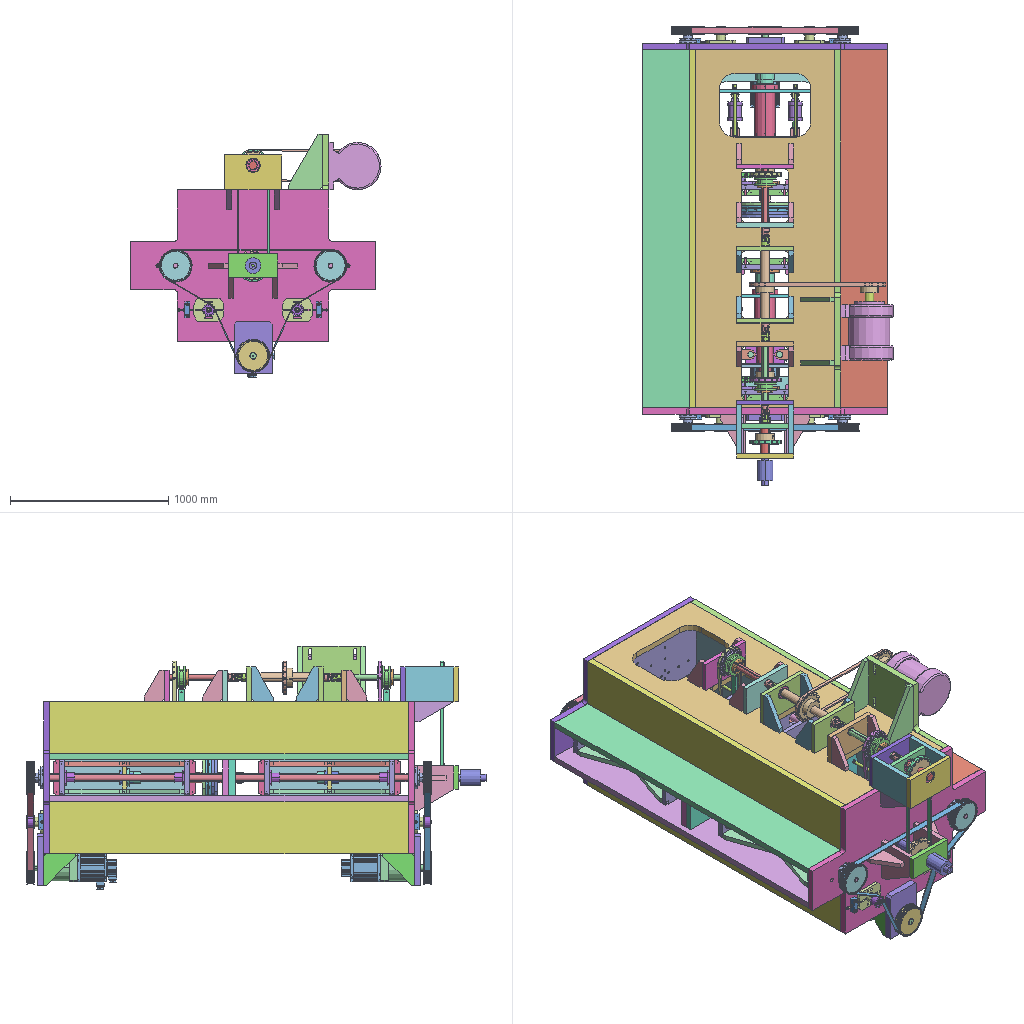Assembly | SolidWorks | 129 different items | 522 placed | box 1583 x 2910 x 1538 mm
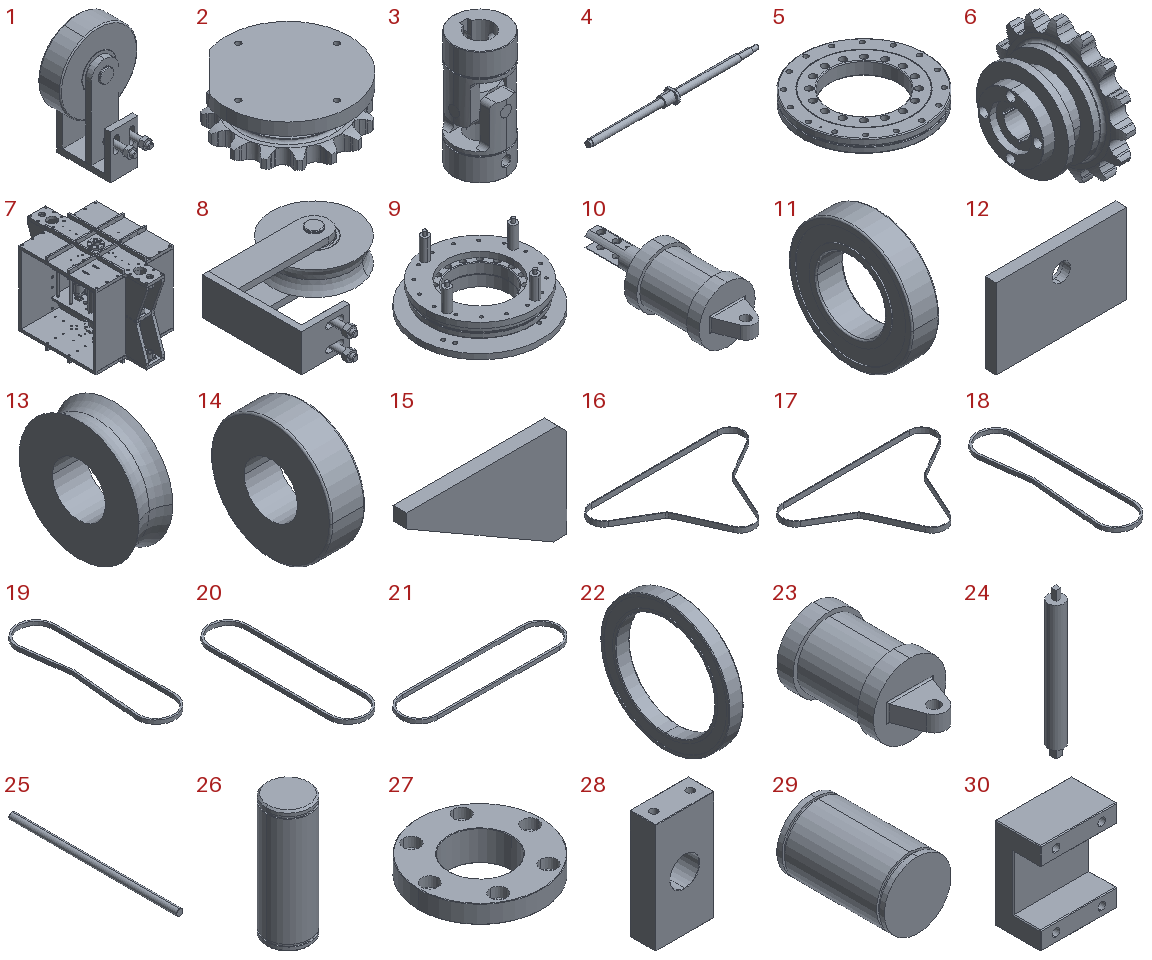Parts list (item | name | quantity | parent item | size | volume | features):
1 | (subassembly) | x2 | - | 140 x 135.4 x 210 mm | 1382662 mm3 | features ReferencePattern 2, LocalLPattern 1
2 | (subassembly) | x2 | - | 200 x 200 x 79.02 mm | 1384453 mm3 | -
3 | (subassembly) | x3 | - | 50 x 50 x 108 mm | 130894 mm3 | -
4 | (subassembly) | x4 | - | 1281 x 110 x 85 mm | 2659708 mm3 | -
5 | (subassembly) | x1 | in 9 | 380 x 380 x 40 mm | 2781012 mm3 | features ReferencePattern 29, CompositeCurve 5, LocalCirPattern 1, MirrorCompFeat 1
6 | (subassembly) | x2 | - | 100.469 x 197.46 x 198.492 mm | 1236352 mm3 | -
7 | (subassembly) | x2 | - | - | 136371359 mm3 | -
8 | (subassembly) | x2 | - | 230 x 244.4 x 70 mm | 814861 mm3 | features ReferencePattern 2, LocalLPattern 1
9 | (subassembly) | x1 | - | 460 x 460 x 195 mm | 7776901 mm3 | features InContextFeatHolder 6, ReferencePattern 3, LocalCirPattern 1
10 | (subassembly) | x4 | in 7 | 90 x 260 x 90 mm | 556632 mm3 | -
11 | - | x4 | - | 20 x 90 x 90 mm | 83545 mm3 | features Fillet 2, Revolution 1
12 | - | x1 | - | 360 x 30 x 220 mm | 2312972 mm3 | features Cut 2, Extrusion 1
13 | - | x2 | in 8 | 40 x 140 x 140 mm | 406899 mm3 | features ICE 1, Revolution 1
14 | - | x4 | in 1 | 40 x 140 x 140 mm | 494239 mm3 | features Fillet 1, ICE 1, Revolution 1
15 | - | x2 | - | 350 x 30 x 214.752 mm | 1362087 mm3 | features Extrusion 1
16 | - | x1 | - | 1186 x 775.76 x 38 mm | 604622 mm3 | features BeltProfileFeature 1, ExtruThin 1
17 | - | x1 | - | 1186 x 775.76 x 38 mm | 604622 mm3 | features BeltProfileFeature 1, ExtruThin 1
18 | - | x1 | - | 203.25 x 838.25 x 20 mm | 376153 mm3 | features BeltProfileFeature 1, ExtruThin 1
19 | - | x1 | - | 203.25 x 838.25 x 20 mm | 376153 mm3 | features BeltProfileFeature 1, ExtruThin 1
20 | - | x1 | - | 203.25 x 838.25 x 20 mm | 375423 mm3 | features BeltProfileFeature 1, ExtruThin 1
21 | - | x1 | - | 863.25 x 208.25 x 20 mm | 385430 mm3 | features BeltProfileFeature 1, ExtruThin 1
22 | - | x4 | in 2 | 7 x 65 x 65 mm | 8944 mm3 | features Fillet 2, Revolution 1
23 | - | x4 | in 10 | 90 x 165 x 90 mm | 446114 mm3 | features ICE 5, Extrusion 1, Fillet 1
24 | - | x1 | - | 50 x 50 x 450 mm | 785743 mm3 | features Extrusion 1, ICE 1, MoveFace 1
25 | - | x16 | in 7 | 20 x 520 x 20 mm | 163347 mm3 | features Chamfer 1, Extrusion 1
26 | - | x8 | in 1, 8 | 25 x 25 x 70 mm | 34175 mm3 | features LibraryFeature 2, RevCut 2, Chamfer 1, Extrusion 1
27 | - | x4 | in 7 | 135 x 135 x 33 mm | 218081 mm3 | features Chamfer 1, CirPattern 1, HoleWzd 1, Revolution 1
28 | - | x4 | in 7 | 80 x 35 x 150 mm | 365960 mm3 | features HoleWzd 2, Chamfer 1, Extrusion 1
29 | - | x8 | in 7 | 40 x 64.4 x 40 mm | 80410 mm3 | features Extrusion 1, MirrorPattern 1, RevCut 1
30 | - | x4 | in 7 | 50 x 30 x 60 mm | 56292 mm3 | features Chamfer 2, Extrusion 1, HoleWzd 1, ICE 1
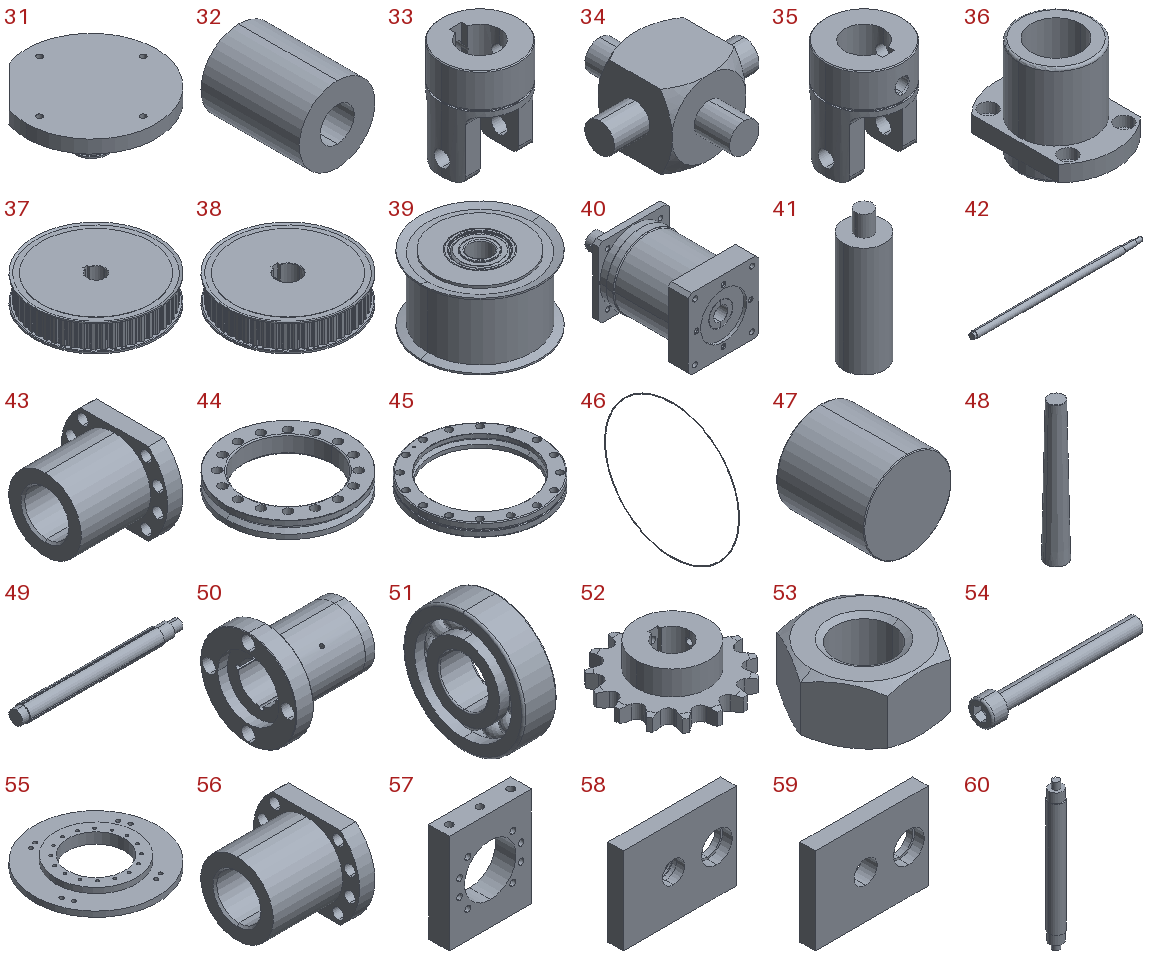31 | - | x2 | in 2 | 200 x 200 x 79.02 mm | 730688 mm3 | features HoleWzd 2, ICE 2, CirPattern 1, Revolution 1
32 | - | x1 | - | 100 x 130 x 100 mm | 814262 mm3 | features Extrusion 1
33 | - | x3 | in 3 | 50 x 50 x 64 mm | 55881 mm3 | features RefAxis 6, ICE 4, 3DProfileFeature 2, RevCut 2, LockFeature 1, Revolution 1
34 | - | x3 | in 3 | 49 x 49 x 25 mm | 19131 mm3 | features RefAxis 3, ICE 2, RevCut 2, 3DProfileFeature 1, Extrusion 1, LockFeature 1
35 | - | x3 | in 3 | 50 x 50 x 64 mm | 55881 mm3 | features ICE 4, RefAxis 3, RevCut 2, 3DProfileFeature 1, LockFeature 1, Revolution 1
36 | - | x8 | in 7 | 66 x 96 x 80 mm | 157671 mm3 | features RevCut 4, ICE 1, LockFeature 1, Revolution 1
37 | - | x4 | - | 210 x 210 x 46.349 mm | 1373265 mm3 | features Revolution 6, ICE 4, RevCut 3, LockFeature 1
38 | - | x2 | - | 210 x 210 x 46.349 mm | 1347722 mm3 | features Revolution 6, ICE 4, RevCut 3, LockFeature 1
39 | - | x4 | - | 80 x 80 x 45 mm | 153277 mm3 | features Revolution 3, LockFeature 1
40 | - | x2 | - | 176.2 x 324.5 x 176 mm | 5934873 mm3 | features ICE 15, CirPattern 7, Fillet 5, Chamfer 4, 3DProfileFeature 1, CombineBodies 1, HoleWzd 1, RefAxis 1, Revolution 1
41 | - | x4 | in 9 | 30 x 30 x 95 mm | 57062 mm3 | features Extrusion 1, HoleWzd 1, ICE 1
42 | - | x4 | in 4 | 1281 x 50 x 50 mm | 2368676 mm3 | features RefAxis 6, 3DProfileFeature 2, ICE 1, LockFeature 1, Revolution 1
43 | - | x4 | in 4 | 88 x 110 x 85 mm | 291032 mm3 | features ICE 9, RefAxis 4, 3DProfileFeature 1, LockFeature 1, RevCut 1, Revolution 1
44 | - | x1 | in 5 | 295 x 295 x 40 mm | 1150106 mm3 | features CirPattern 1, Extrusion 1, Fillet 1, HoleWzd 1, ICE 1, MirrorPattern 1, RefAxis 1, RevCut 1
45 | - | x1 | in 5 | 380 x 380 x 40 mm | 1589572 mm3 | features ICE 4, CirPattern 2, Extrusion 1, Fillet 1, HoleWzd 1, MirrorPattern 1, RefAxis 1, RevCut 1
46 | - | x2 | in 5 | 0.4 x 296.6 x 296.6 mm | 561.725 mm3 | features Revolution 1
47 | - | x29 | in 5 | 12 x 12 x 12 mm | 1357 mm3 | features Fillet 1, RefAxis 1, Revolution 1
48 | - | x1 | in 5 | 5.996 x 5.996 x 40 mm | 857.367 mm3 | features Extrusion 1, Fillet 1
49 | - | x1 | - | 419 x 40 x 40 mm | 488497 mm3 | features ICE 6, RefAxis 3, 3DProfileFeature 1, LockFeature 1, Revolution 1
50 | - | x2 | in 6 | 100 x 100 x 100 mm | 246930 mm3 | features RevCut 6, Revolution 5, RefAxis 3, ICE 2, 3DProfileFeature 1, LockFeature 1
51 | - | x8 | in 1, 8 | 17 x 62 x 62 mm | 31055 mm3 | features Revolution 3, Fillet 2, CirPattern 1
52 | - | x6 | in 7 | 201.53 x 200.494 x 63 mm | 849751 mm3 | features BaseBody 1
53 | - | x100 | in 7 | 18.475 x 16 x 8.4 mm | 1367 mm3 | features RevCut 2, Chamfer 1, Extrusion 1, LPattern 1
54 | - | x4 | - | 100 x 16 x 16 mm | 8745 mm3 | features Fillet 2, RevCut 2, Boss 1, Chamfer 1, Cut 1, Extrusion 1, LPattern 1
55 | - | x1 | in 9 | 460 x 460 x 40 mm | 3276881 mm3 | features HoleWzd 2, ICE 2, CirPattern 1, Extrusion 1
56 | - | x4 | in 7 | 88 x 110 x 85 mm | 291032 mm3 | features ICE 9, RefAxis 4, 3DProfileFeature 1, LockFeature 1, RevCut 1, Revolution 1
57 | - | x4 | in 7 | 120 x 30 x 145 mm | 363114 mm3 | features HoleWzd 2, Extrusion 1, MirrorPattern 1
58 | - | x2 | - | 293 x 40 x 225 mm | 2341161 mm3 | features Cut 3, ICE 2, Extrusion 1
59 | - | x2 | - | 293 x 40 x 225 mm | 2340512 mm3 | features Cut 3, Extrusion 1
60 | - | x1 | - | 55 x 55 x 548.93 mm | 1170773 mm3 | features Cut 2, ICE 1, Revolution 1
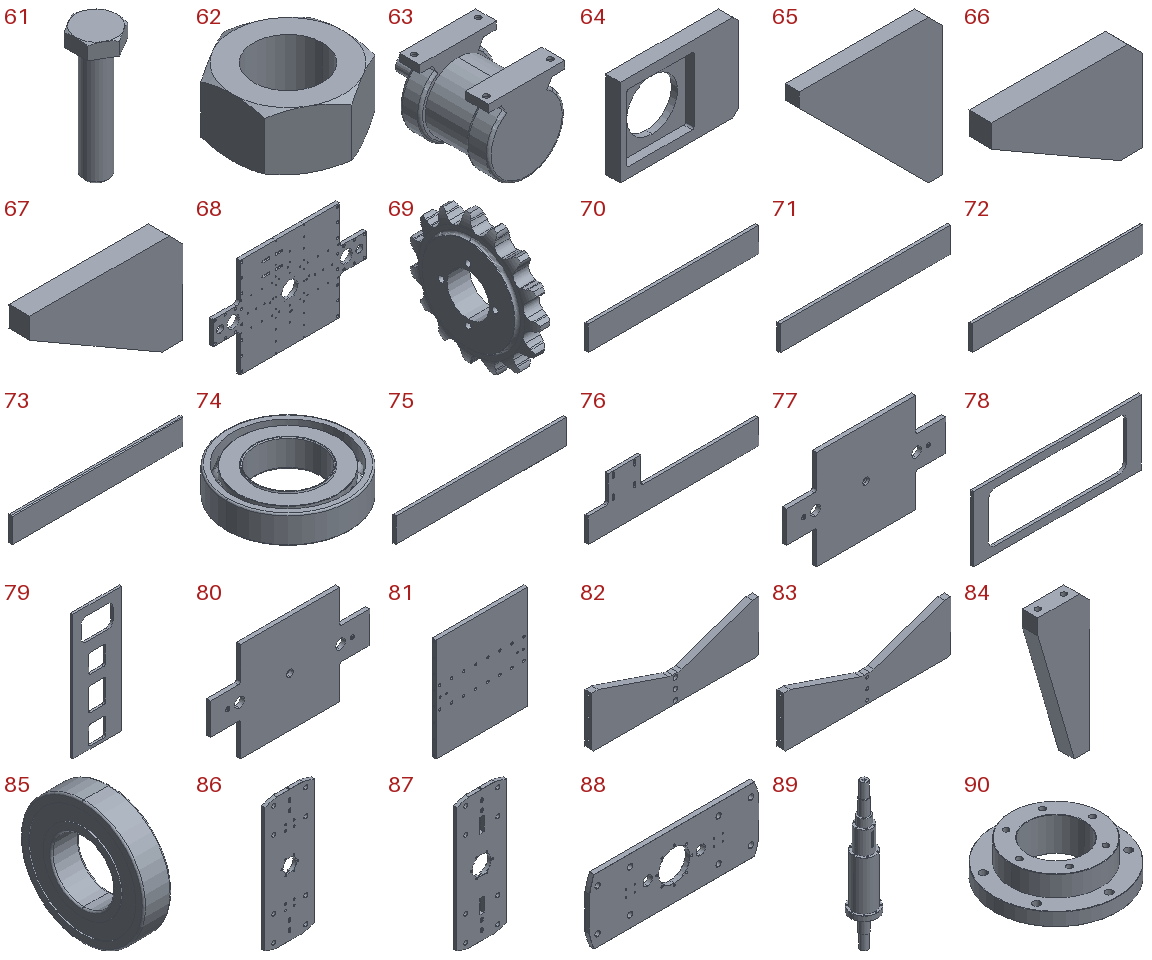61 | - | x9 | in 1, 8 | 16 x 18.475 x 51.2 mm | 4858 mm3 | features ICE 3, Chamfer 1, Extrusion 1, Fillet 1, RefAxis 1
62 | - | x10 | in 1, 8 | 16 x 18.475 x 8.4 mm | 1194 mm3 | features ICE 3, Extrusion 1, RefAxis 1
63 | - | x1 | - | 300 x 490 x 330 mm | 24115520 mm3 | features ICE 4, Extrusion 1, Fillet 1, HoleWzd 1
64 | - | x2 | - | 325 x 40 x 240 mm | 2062624 mm3 | features Cut 2, Chamfer 1, Extrusion 1, Fillet 1
65 | - | x4 | - | 200 x 20 x 200 mm | 472000 mm3 | features Extrusion 1
66 | - | x8 | - | 200 x 30 x 128.15 mm | 512616 mm3 | features Extrusion 1
67 | - | x4 | - | 220 x 30 x 139.697 mm | 603362 mm3 | features Extrusion 1
68 | - | x4 | in 7 | 1326 x 30 x 860 mm | 23495138 mm3 | features HoleWzd 7, MirrorPattern 4, Cut 3, DelFace 2, ICE 2, Cavity 1, CirPattern 1, Extrusion 1, Fillet 1, MoveFace 1
69 | - | x2 | in 6 | 34.469 x 197.46 x 198.492 mm | 621986 mm3 | features ICE 3, CirPattern 1, Cut 1, HoleWzd 1, RefAxis 1, Revolution 1
70 | - | x3 | - | 2266 x 40 x 327.5 mm | 29684600 mm3 | features Extrusion 1
71 | - | x1 | - | 2266 x 40 x 333 mm | 30069820 mm3 | features Chamfer 1, Extrusion 1
72 | - | x1 | - | 2266 x 40 x 333 mm | 30069820 mm3 | features Chamfer 1, Extrusion 1
73 | - | x1 | - | 2266 x 40 x 333 mm | 30069820 mm3 | features Chamfer 1, Extrusion 1
74 | - | x8 | in 7 | 85 x 85 x 19 mm | 41492 mm3 | features Revolution 5, Fillet 2, CirPattern 1, LockFeature 1, RefAxis 1
75 | - | x1 | - | 2266 x 40 x 333 mm | 30069820 mm3 | features Chamfer 1, Extrusion 1
76 | - | x1 | - | 2266 x 40 x 677.5 mm | 35483230 mm3 | features Cut 1, Extrusion 1, Fillet 1, ICE 1
77 | - | x1 | - | 1546 x 40 x 960 mm | 43281864 mm3 | features Cut 4, MirrorPattern 2, Extrusion 1, Fillet 1, HoleWzd 1
78 | - | x1 | - | 2266 x 40 x 880 mm | 29351363 mm3 | features Cut 1, Extrusion 1, Fillet 1
79 | - | x1 | - | 880 x 40 x 2266 mm | 57536483 mm3 | features Cut 4, Fillet 2, Extrusion 1
80 | - | x1 | - | 1546 x 40 x 960 mm | 43282780 mm3 | features Cut 3, MirrorPattern 2, Extrusion 1, Fillet 1, HoleWzd 1
81 | - | x4 | in 7 | 763 x 30 x 860 mm | 19515474 mm3 | features HoleWzd 4, Extrusion 1
82 | - | x4 | in 7 | 763 x 30 x 233 mm | 4012044 mm3 | features HoleWzd 4, Chamfer 1, Extrusion 1, Fillet 1, ICE 1
83 | - | x4 | in 7 | 763 x 30 x 233 mm | 4012044 mm3 | features HoleWzd 4, Chamfer 1, Extrusion 1, Fillet 1, ICE 1
84 | - | x8 | in 7 | 100 x 30 x 270 mm | 537159 mm3 | features HoleWzd 2, Extrusion 1
85 | - | x4 | - | 18 x 80 x 80 mm | 64676 mm3 | features Fillet 2, Revolution 1
86 | - | x2 | in 7 | 280 x 20 x 735 mm | 3763100 mm3 | features HoleWzd 5, MirrorPattern 5, Cut 4, ICE 3, Chamfer 1, Extrusion 1
87 | - | x2 | in 7 | 280 x 20 x 735 mm | 3611529 mm3 | features Cut 5, HoleWzd 4, MirrorPattern 4, Fillet 2, ICE 2, Chamfer 1, Extrusion 1
88 | - | x2 | in 7 | 735 x 20 x 280 mm | 3653235 mm3 | features HoleWzd 3, MirrorPattern 3, ICE 2, Chamfer 1, Cut 1, Extrusion 1
89 | - | x2 | in 7 | 165 x 165 x 903 mm | 6812270 mm3 | features Chamfer 4, CirPattern 3, HoleWzd 3, ICE 2, Cut 1, Revolution 1
90 | - | x4 | in 7 | 185 x 185 x 51 mm | 661113 mm3 | features CirPattern 2, HoleWzd 2, Chamfer 1, Revolution 1
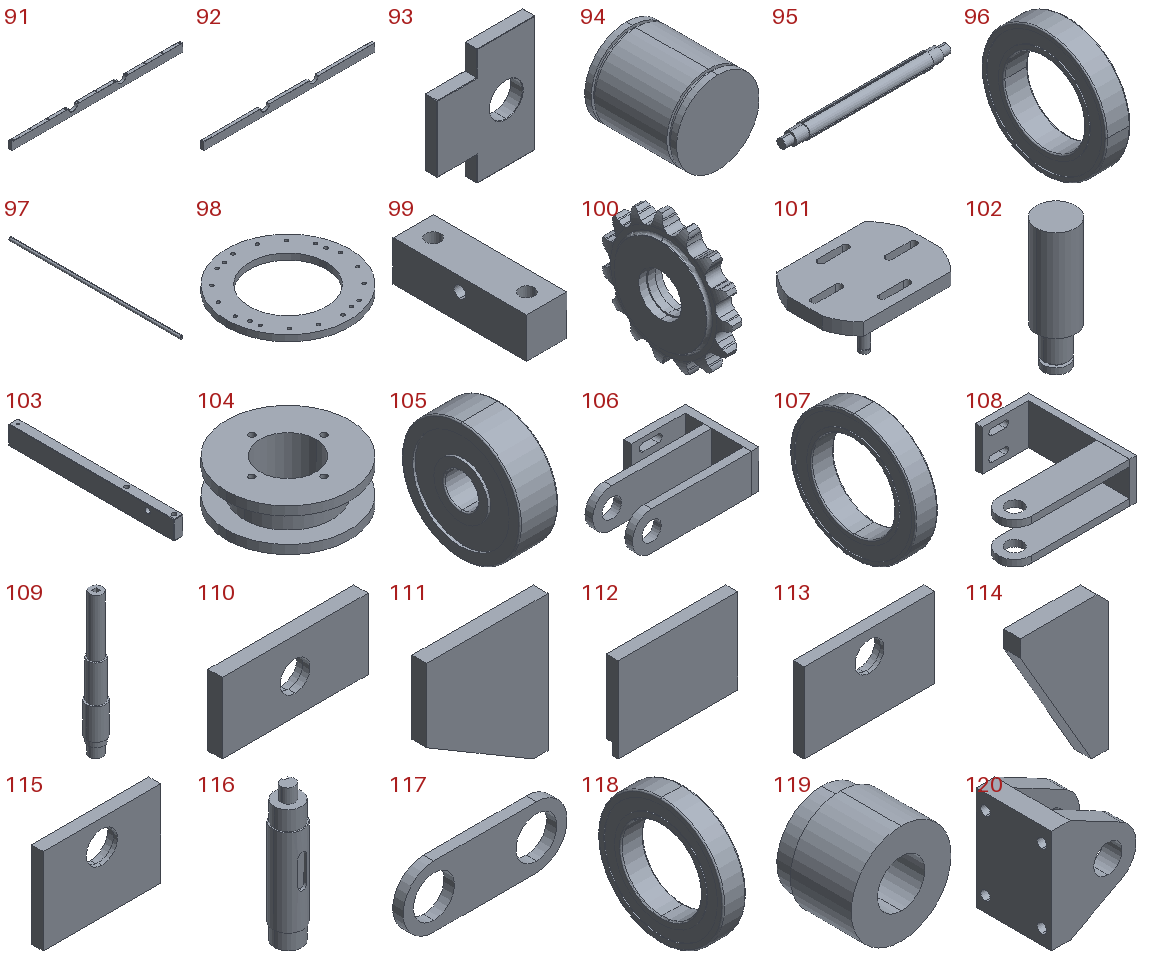91 | - | x8 | in 7 | 860 x 15 x 40 mm | 485456 mm3 | features Chamfer 3, Extrusion 1, HoleWzd 1, ICE 1
92 | - | x8 | in 7 | 860 x 15 x 40 mm | 485456 mm3 | features Chamfer 3, Extrusion 1, HoleWzd 1, ICE 1
93 | - | x4 | in 7 | 118 x 15 x 140 mm | 185579 mm3 | features Chamfer 1, Extrusion 1
94 | - | x4 | in 7 | 40 x 44.4 x 40 mm | 55277 mm3 | features Extrusion 1, MirrorPattern 1, RevCut 1
95 | - | x1 | - | 462 x 40 x 40 mm | 516055 mm3 | features ICE 7, RefAxis 3, 3DProfileFeature 1, LockFeature 1, MirrorPattern 1, MoveFace 1, Revolution 1
96 | - | x2 | - | 12 x 62 x 62 mm | 20018 mm3 | features Fillet 2, Revolution 1
97 | - | x2 | - | 40 x 2286 x 40 mm | 2864710 mm3 | features HoleWzd 2, Extrusion 1
98 | - | x1 | in 9 | 400 x 400 x 20 mm | 1490760 mm3 | features CirPattern 2, HoleWzd 2, Extrusion 1, ICE 1
99 | - | x4 | - | 30 x 100 x 30 mm | 79088 mm3 | features HoleWzd 2, Extrusion 1
100 | - | x2 | in 2 | 34.469 x 197.46 x 198.492 mm | 635877 mm3 | features ICE 4, CirPattern 1, Cut 1, MirrorPattern 1, RefAxis 1, Revolution 1
101 | - | x4 | - | 192 x 141 x 111 mm | 573691 mm3 | features ICE 2, MirrorPattern 2, Revolution 1
102 | - | x2 | - | 12.8 x 12.8 x 42 mm | 4440 mm3 | features Revolution 1
103 | - | x2 | - | 20 x 350 x 40 mm | 265293 mm3 | features HoleWzd 3, Chamfer 1, Extrusion 1, ICE 1
104 | - | x2 | in 6 | 140 x 140 x 48 mm | 367436 mm3 | features HoleWzd 2, Revolution 1
105 | - | x2 | - | 9 x 28 x 28 mm | 4750 mm3 | features RefAxis 3, Revolution 1
106 | - | x2 | in 1 | 165 x 96.4 x 50 mm | 217447 mm3 | features MoveFace 6, ICE 4, MoveCopyBody 2, Extrusion 1, MirrorSolid 1, Split 1
107 | - | x2 | - | 12 x 68 x 68 mm | 23116 mm3 | features Fillet 2, Revolution 1
108 | - | x2 | in 8 | 185 x 164.4 x 62 mm | 299575 mm3 | features ICE 3, Extrusion 1, MirrorSolid 1, Split 1
109 | - | x1 | - | 65 x 65 x 493 mm | 970539 mm3 | features ICE 2, Chamfer 1, Revolution 1
110 | - | x1 | - | 310 x 30 x 150 mm | 1293021 mm3 | features Cut 2, Extrusion 1
111 | - | x2 | - | 250 x 30 x 280 mm | 1671000 mm3 | features Extrusion 1
112 | - | x2 | - | 308.5 x 30 x 220 mm | 1897275 mm3 | features Cut 1, Extrusion 1
113 | - | x1 | - | 360 x 30 x 220 mm | 2198500 mm3 | features Cut 2, Extrusion 1
114 | - | x2 | - | 155.862 x 30 x 248 mm | 742046 mm3 | features Extrusion 1
115 | - | x1 | - | 300 x 30 x 220 mm | 1802500 mm3 | features Cut 2, Extrusion 1
116 | - | x1 | - | 55 x 55 x 251.5 mm | 515825 mm3 | features Cut 1, ICE 1, Revolution 1
117 | - | x16 | in 7 | 160 x 10 x 60 mm | 63142 mm3 | features Extrusion 1
118 | - | x4 | - | 10 x 55 x 55 mm | 13514 mm3 | features Fillet 2, Revolution 1
119 | - | x2 | in 7 | 118 x 94 x 118 mm | 750005 mm3 | features Extrusion 1, ICE 1
120 | - | x4 | in 7 | 45 x 40 x 55 mm | 42289 mm3 | features Chamfer 1, Extrusion 1, HoleWzd 1, ICE 1
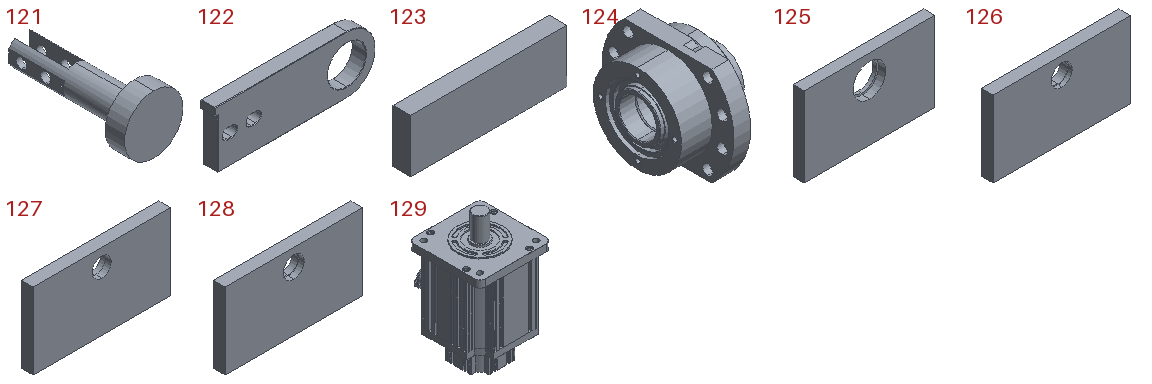121 | - | x4 | in 10 | 60 x 135 x 60 mm | 110518 mm3 | features ICE 3, HoleWzd 2, Extrusion 1
122 | - | x4 | in 7 | 168 x 15 x 60 mm | 119877 mm3 | features Chamfer 1, Extrusion 1, ICE 1
123 | - | x4 | in 7 | 44 x 5 x 15 mm | 3300 mm3 | features Extrusion 1
124 | - | x4 | - | 86 x 142 x 106 mm | 475751 mm3 | features ICE 14, Revolution 8, RefAxis 5, CirPattern 4, LPattern 1, RevCut 1
125 | - | x2 | - | 360 x 30 x 220 mm | 2198500 mm3 | features Cut 2, Extrusion 1
126 | - | x1 | - | 360 x 30 x 200 mm | 2096972 mm3 | features Cut 2, Extrusion 1
127 | - | x1 | - | 360 x 30 x 200 mm | 2095104 mm3 | features Cut 2, Extrusion 1
128 | - | x1 | - | 360 x 30 x 200 mm | 2095104 mm3 | features Cut 2, Extrusion 1
129 | - | x2 | - | 180 x 228 x 314 mm | 6100374 mm3 | features ICE 33, Fillet 11, MirrorPattern 7, CirPattern 5, Extrusion 3, Revolution 3, Chamfer 2, Sweep 2, PLine 1
Mates (type | each side: item.copy, entity, surface, feature), first 345 of 680 lines:
In the top assembly
Coincident | 80.1 face plane Boss-Extrude 1 | 76.1 face plane Boss-Extrude 1 | 2 times
Coincident | 80.1 face plane Boss-Extrude 1 | 70.1 face plane Boss-Extrude 1 | 3 times
Coincident | 80.1 face plane Boss-Extrude 1 | 70.2 face plane Boss-Extrude 1 | 3 times
Coincident | 80.1 face plane Boss-Extrude 1 | 70.3 face plane Boss-Extrude 1 | 3 times
Coincident | 80.1 face plane Boss-Extrude 1 | 75.1 face plane Boss-Extrude 1 | 3 times
Coincident | 80.1 face plane Boss-Extrude 1 | 71.1 face plane Boss-Extrude 1 | 3 times
Coincident | 80.1 face plane Boss-Extrude 1 | 72.1 face plane Boss-Extrude 1 | 3 times
Coincident | 80.1 face plane Boss-Extrude 1 | 73.1 face plane Boss-Extrude 1 | 3 times
Width | 80.1 face plane Boss-Extrude 1 | 80.1 face plane Boss-Extrude 1 | 68.1 face plane Boss-Extrude 1 | 68.1 face plane Boss-Extrude 1
Width | 70.1 face plane Boss-Extrude 1 | 70.2 face plane Boss-Extrude 1 | 81.1 face plane Boss-Extrude 1 | 81.2 face plane Boss-Extrude 1
Concentric | 36.1 face cylinder Revolve 1 | 97.1 face cylinder Boss-Extrude 1
Coincident | 80.1 face plane Cut-Extrude 1 | 97.1 face plane Boss-Extrude 1
Concentric | 36.2 face cylinder Revolve 1 | 97.2 face cylinder Boss-Extrude 1
Coincident | 80.1 face plane Mirror 1 | 97.2 face plane Boss-Extrude 1
Concentric | 56.1 face cylinder Revolve 1 | 124.1 face cylinder Revolve 1
Parallel | 80.1 face plane Boss-Extrude 1 | 124.1 face plane Cut-Extrude 1
Coincident | 80.1 face plane Boss-Extrude 1 | 124.1 face plane Revolve 1
Concentric | 80.1 face cylinder Mirror 2 | 124.2 face cylinder Revolve 1
Coincident | 80.1 face plane Boss-Extrude 1 | 124.2 face plane Revolve 1
Coincident | 71.1 face plane Boss-Extrude 1 | 58.1 face plane Boss-Extrude 1
Concentric | 58.1 face cylinder Cut-Extrude 1 | 85.1 face cylinder Revolve1
Coincident | 58.1 face plane Cut-Extrude 1 | 85.1 face plane Revolve1
Coincident | 72.1 face plane Boss-Extrude 1 | 58.2 face plane Boss-Extrude 1
Coincident | 58.1 face plane Boss-Extrude 1 | 58.2 face plane Boss-Extrude 1
DistanceDim | 58.2 face plane Boss-Extrude 1 | 80.1 face plane Boss-Extrude 1
Concentric | 58.2 face cylinder Cut-Extrude 1 | 85.2 face cylinder Revolve1
Coincident | 58.2 face plane Cut-Extrude 1 | 85.2 face plane Revolve1
Coincident | 75.1 face plane Boss-Extrude 1 | 59.1 face plane Boss-Extrude 1
Coincident | 58.1 face plane Boss-Extrude 1 | 59.1 face plane Boss-Extrude 1
Concentric | 59.1 face cylinder Cut-Extrude 1 | 85.3 face cylinder Revolve1
Coincident | 59.1 face plane Cut-Extrude 1 | 85.3 face plane Revolve1
Coincident | 75.1 face plane Boss-Extrude 1 | 77.1 face plane Boss-Extrude 1 | 2 times
Coincident | 70.2 face plane Boss-Extrude 1 | 77.1 face plane Boss-Extrude 1
Concentric | 77.1 face cylinder Cut-Extrude 2 | 124.3 face cylinder Revolve 1
Coincident | 77.1 face plane Boss-Extrude 1 | 124.3 face plane Revolve 1
Parallel | 77.1 face plane Boss-Extrude 1 | 124.3 face plane Cut-Extrude 1
Concentric | 77.1 face cylinder Mirror 2 | 124.4 face cylinder Revolve 1
Coincident | 77.1 face plane Boss-Extrude 1 | 124.4 face plane Revolve 1
Parallel | 77.1 face plane Boss-Extrude 1 | 124.4 face plane Cut-Extrude 1
Width | 76.1 face plane Boss-Extrude 1 | 70.3 face plane Boss-Extrude 1 | 81.3 face plane Boss-Extrude 1 | 81.4 face plane Boss-Extrude 1
Width | 72.1 face plane Boss-Extrude 1 | 73.1 face plane Boss-Extrude 1 | 82.1 face plane Boss-Extrude 1 | 83.1 face plane Boss-Extrude 1
Coincident | 70.1 face plane Boss-Extrude 1 | 78.1 face plane Boss-Extrude 1
Coincident | 70.2 face plane Boss-Extrude 1 | 78.1 face plane Boss-Extrude 1
Coincident | 80.1 face plane Boss-Extrude 1 | 78.1 face plane Boss-Extrude 1
Coincident | 70.1 face plane Boss-Extrude 1 | 58.2 face plane Boss-Extrude 1
Coincident | 70.2 face plane Boss-Extrude 1 | 58.1 face plane Boss-Extrude 1
Coincident | 70.3 face plane Boss-Extrude 1 | 59.1 face plane Boss-Extrude 1
Concentric | 56.1 face cylinder Revolve 1 | 42.1 face cylinder Revolve 1
Coincident | 124.1 face plane Revolve 4 | 42.1 face plane Revolve 1
Concentric | 56.2 face cylinder Revolve 1 | 42.2 face cylinder Revolve 1
Coincident | 124.2 face plane Revolve 4 | 42.2 face plane Revolve 1
Concentric | 56.3 face cylinder Revolve 1 | 42.3 face cylinder Revolve 1
Coincident | 124.4 face plane Revolve 4 | 42.3 face plane Revolve 1
Concentric | 56.4 face cylinder Revolve 1 | 42.4 face cylinder Revolve 1
Coincident | 124.3 face plane Revolve 4 | 42.4 face plane Revolve 1
Concentric | 42.4 face cylinder Revolve 1 | 37.1 face cylinder Cut-Revolve 1
Coincident | 42.4 face plane Revolve 1 | 37.1 face plane Revolve 1
Concentric | 42.3 face cylinder Revolve 1 | 37.2 face cylinder Cut-Revolve 1
Coincident | 42.3 face plane Revolve 1 | 37.2 face plane Revolve 1
Concentric | 42.1 face cylinder Revolve 1 | 37.3 face cylinder Cut-Revolve 1
Coincident | 42.1 face plane Revolve 1 | 37.3 face plane Revolve 1
Concentric | 42.2 face cylinder Revolve 1 | 37.4 face cylinder Cut-Revolve 1
Coincident | 42.2 face plane Revolve 1 | 37.4 face plane Revolve 1
Concentric | 129.1 face cylinder Revolve 1 | 40.1 face cylinder Cut-Extrude 5
Coincident | 129.1 face plane Boss-Extrude 1 | 40.1 face plane Boss-Extrude 1
Width | 80.1 face plane Boss-Extrude 1 | 80.1 face plane Boss-Extrude 1 | 40.1 face plane Boss-Extrude 7 | 40.1 face plane Boss-Extrude 7
Concentric | 129.2 face cylinder Revolve 1 | 40.2 face cylinder Cut-Extrude 5
Coincident | 129.2 face plane Boss-Extrude 1 | 40.2 face plane Boss-Extrude 1
Coincident | 80.1 face plane Boss-Extrude 1 | 64.1 face plane Boss-Extrude 1
DistanceDim | 64.1 face plane Boss-Extrude 1 | 80.1 face plane Boss-Extrude 1
Width | 80.1 face plane Boss-Extrude 1 | 80.1 face plane Boss-Extrude 1 | 64.1 face plane Boss-Extrude 1 | 64.1 face plane Boss-Extrude 1
Coincident | 40.1 face plane Revolve 1 | 64.1 face plane Cut-Extrude 1
Coincident | 77.1 face plane Boss-Extrude 1 | 64.2 face plane Boss-Extrude 1
DistanceDim | 64.2 face plane Boss-Extrude 1 | 77.1 face plane Boss-Extrude 1
Width | 77.1 face plane Boss-Extrude 1 | 77.1 face plane Boss-Extrude 1 | 64.2 face plane Boss-Extrude 1 | 64.2 face plane Boss-Extrude 1
Coincident | 40.2 face plane Revolve 1 | 64.2 face plane Cut-Extrude 1
Width | 70.1 face plane Boss-Extrude 1 | 70.2 face plane Boss-Extrude 1 | 40.2 face plane Boss-Extrude 1 | 40.2 face plane Boss-Extrude 1
Coincident | 64.1 face plane Boss-Extrude 1 | 65.1 face plane Boss-Extrude 1 | 2 times
Coincident | 78.1 face plane Boss-Extrude 1 | 65.1 face plane Boss-Extrude 1
Coincident | 64.1 face plane Boss-Extrude 1 | 65.2 face plane Boss-Extrude 1 | 2 times
Coincident | 78.1 face plane Boss-Extrude 1 | 65.2 face plane Boss-Extrude 1
Coincident | 64.2 face plane Boss-Extrude 1 | 65.3 face plane Boss-Extrude 1 | 2 times
Coincident | 78.1 face plane Boss-Extrude 1 | 65.3 face plane Boss-Extrude 1
Coincident | 64.2 face plane Boss-Extrude 1 | 65.4 face plane Boss-Extrude 1 | 2 times
Coincident | 78.1 face plane Boss-Extrude 1 | 65.4 face plane Boss-Extrude 1
Concentric | 40.1 face cylinder Revolve 1 | 38.1 face cylinder Cut-Revolve 1
Coincident | 37.4 face plane Revolve 1 | 38.1 face plane Revolve 1
Concentric | 40.2 face cylinder Revolve 1 | 38.2 face cylinder Cut-Revolve 1
Coincident | 37.2 face plane Revolve 1 | 38.2 face plane Revolve 1
Coincident | 80.1 face plane Boss-Extrude 1 | 101.1 face plane Revolve 1
DistanceDim | 101.1 plane | 80.1 face plane Boss-Extrude 1 | 2 times
Coincident | 80.1 face plane Boss-Extrude 1 | 101.2 face plane Revolve 1
DistanceDim | 101.2 plane | 80.1 face plane Boss-Extrude 1 | 2 times
Concentric | 101.1 face cylinder Revolve 1 | 39.1 face cylinder Revolve 3
Coincident | 101.1 face plane Revolve 1 | 39.1 face plane Revolve 2
Concentric | 101.2 face cylinder Revolve 1 | 39.2 face cylinder Revolve 3
Coincident | 101.2 face plane Revolve 1 | 39.2 face plane Revolve 2
Coincident | 77.1 face plane Boss-Extrude 1 | 101.3 face plane Revolve 1
Coincident | 77.1 face plane Boss-Extrude 1 | 101.4 face plane Revolve 1
Concentric | 101.3 face cylinder Revolve 1 | 39.3 face cylinder Revolve 2
Coincident | 101.3 face plane Revolve 1 | 39.3 face plane Revolve 3
Concentric | 101.4 face cylinder Revolve 1 | 39.4 face cylinder Revolve 2
Coincident | 101.4 face plane Revolve 1 | 39.4 face plane Revolve 3
Coincident | 80.1 face plane Boss-Extrude 1 | 99.1 face plane Boss-Extrude 1
DistanceDim | 99.1 face plane Boss-Extrude 1 | 101.2 face plane Cut-Extrude 2
Width | 101.2 face plane Cut-Extrude 2 | 101.2 face plane Cut-Extrude 2 | 99.1 face plane Boss-Extrude 1 | 99.1 face plane Boss-Extrude 1
Width | 101.1 face plane Cut-Extrude 2 | 101.1 face plane Cut-Extrude 2 | 99.2 face plane Boss-Extrude 1 | 99.2 face plane Boss-Extrude 1
DistanceDim | 99.2 face plane Boss-Extrude 1 | 101.1 face plane Cut-Extrude 2
Coincident | 80.1 face plane Boss-Extrude 1 | 99.2 face plane Boss-Extrude 1
Coincident | 77.1 face plane Boss-Extrude 1 | 99.3 face plane Boss-Extrude 1
Coincident | 77.1 face plane Boss-Extrude 1 | 99.4 face plane Boss-Extrude 1
Concentric | 99.1 face cylinder M10 Tapped Hole 1 | 54.1 face cylinder BaseBody
Concentric | 99.2 face cylinder M10 Tapped Hole 1 | 54.2 face cylinder BaseBody
Concentric | 99.4 face cylinder M10 Tapped Hole 1 | 54.3 face cylinder BaseBody
Concentric | 99.3 face cylinder M10 Tapped Hole 1 | 54.4 face cylinder BaseBody
Coincident | 101.2 face plane Cut-Extrude 2 | 54.1 edge
Coincident | 101.1 face plane Cut-Extrude 2 | 54.2 face plane BaseBody
Concentric | 54.1 face cylinder BaseBody | 53.1 face cone EndChamfer
Coincident | 99.1 face plane Boss-Extrude 1 | 53.1 face plane BaseNut
Concentric | 99.2 face cylinder M10 Tapped Hole 1 | 53.2 face cone EndChamfer
Coincident | 99.2 face plane Boss-Extrude 1 | 53.2 face plane BaseNut
Concentric | 99.3 face cylinder M10 Tapped Hole 1 | 53.3 face cone EndChamfer
Coincident | 99.3 face plane Boss-Extrude 1 | 53.3 face plane BaseNut
Concentric | 54.3 face cylinder BaseBody | 53.4 face cone EndChamfer
Coincident | 99.4 face plane Boss-Extrude 1 | 53.4 face plane BaseNut
DistanceDim | 101.3 face plane Cut-Extrude 2 | 77.1 face plane Boss-Extrude 1 | 2 times
Width | 101.3 face plane Cut-Extrude 2 | 101.3 face plane Cut-Extrude 2 | 99.3 face plane Boss-Extrude 1 | 99.3 face plane Boss-Extrude 1
Coincident | 101.3 face plane Cut-Extrude 2 | 54.4 face plane BaseBody
DistanceDim | 99.3 face plane Boss-Extrude 1 | 101.3 face plane Cut-Extrude 2
DistanceDim | 101.4 face plane Cut-Extrude 2 | 77.1 face plane Boss-Extrude 1 | 2 times
Width | 101.4 face plane Cut-Extrude 2 | 101.4 face plane Cut-Extrude 2 | 99.4 face plane Boss-Extrude 1 | 99.4 face plane Boss-Extrude 1
DistanceDim | 101.4 face plane Cut-Extrude 2 | 99.4 face plane Boss-Extrude 1
Coincident | 101.4 face plane Cut-Extrude 2 | 54.3 face plane BaseBody
Width | 72.1 face plane Boss-Extrude 1 | 73.1 face plane Boss-Extrude 1 | 59.2 face plane Boss-Extrude 1 | 59.2 face plane Boss-Extrude 1
Coincident | 76.1 face plane Boss-Extrude 1 | 59.2 face plane Boss-Extrude 1
Coincident | 58.2 face plane Boss-Extrude 1 | 59.2 face plane Boss-Extrude 1
Concentric | 58.2 face cylinder Cut-Extrude 4 | 96.1 face cylinder Revolve1
Coincident | 58.2 face plane Cut-Extrude 4 | 96.1 face plane Revolve1
Concentric | 58.1 face cylinder Cut-Extrude 4 | 96.2 face cylinder Revolve1
Coincident | 58.1 face plane Cut-Extrude 4 | 96.2 face plane Revolve1
Coincident | 76.1 face plane Boss-Extrude 1 | 79.1 face plane Boss-Extrude 1 | 2 times
Coincident | 80.1 face plane Boss-Extrude 1 | 79.1 face plane Boss-Extrude 1
Width | 77.1 face plane Boss-Extrude 1 | 77.1 face plane Boss-Extrude 1 | 110.1 face plane Boss-Extrude 1 | 110.1 face plane Boss-Extrude 1 | 2 times
Coincident | 111.1 face plane Boss-Extrude 1 | 110.1 face plane Boss-Extrude 1 | 3 times
Coincident | 77.1 face plane Boss-Extrude 1 | 111.1 face plane Boss-Extrude 1
Coincident | 110.1 face plane Boss-Extrude 1 | 111.2 face plane Boss-Extrude 1 | 2 times
Coincident | 77.1 face plane Boss-Extrude 1 | 111.2 face plane Boss-Extrude 1
Concentric | 77.1 face cylinder Cut-Extrude 4 | 107.1 face cylinder Revolve1
Coincident | 77.1 face plane Cut-Extrude 4 | 107.1 face plane Revolve1
Coincident | 110.1 face plane Cut-Extrude 2 | 107.2 face plane Revolve1
Concentric | 110.1 face cylinder Cut-Extrude 2 | 107.2 face cylinder Revolve1
Concentric | 107.2 face cylinder Revolve1 | 109.1 face cylinder Revolve 1
Coincident | 107.2 face plane Revolve1 | 109.1 face plane Revolve 1
Concentric | 109.1 face cylinder Revolve 1 | 52.1 face cylinder 输入1
DistanceDim | 52.1 face plane 输入1 | 110.1 face plane Boss-Extrude 1
Coincident | 109.1 face plane Cut-Extrude 2 | 52.1 face plane 输入1
Width | 70.2 face plane Boss-Extrude 1 | 70.1 face plane Boss-Extrude 1 | 126.1 face plane Boss-Extrude 1 | 126.1 face plane Boss-Extrude 1
Width | 70.1 face plane Boss-Extrude 1 | 70.2 face plane Boss-Extrude 1 | 127.1 face plane Boss-Extrude 1 | 127.1 face plane Boss-Extrude 1
Coincident | 76.1 face plane Boss-Extrude 1 | 127.1 face plane Boss-Extrude 1
Width | 76.1 face plane Boss-Extrude 1 | 70.3 face plane Boss-Extrude 1 | 128.1 face plane Boss-Extrude 1 | 128.1 face plane Boss-Extrude 1
Coincident | 76.1 face plane Boss-Extrude 1 | 128.1 face plane Boss-Extrude 1
Width | 70.3 face plane Boss-Extrude 1 | 76.1 face plane Boss-Extrude 1 | 12.1 face plane Boss-Extrude 1 | 12.1 face plane Boss-Extrude 1
Coincident | 76.1 face plane Boss-Extrude 1 | 12.1 face plane Boss-Extrude 1
Coincident | 76.1 face plane Boss-Extrude 1 | 126.1 face plane Boss-Extrude 1
Coincident | 126.1 face plane Cut-Extrude 2 | 118.1 face plane Revolve1
Concentric | 126.1 face cylinder Cut-Extrude 2 | 118.1 face cylinder Revolve1
DistanceDim | 127.1 face plane Boss-Extrude 1 | 80.1 face plane Boss-Extrude 1
DistanceDim | 126.1 face plane Boss-Extrude 1 | 80.1 face plane Boss-Extrude 1
DistanceDim | 128.1 face plane Boss-Extrude 1 | 77.1 face plane Boss-Extrude 1
DistanceDim | 12.1 face plane Boss-Extrude 1 | 77.1 face plane Boss-Extrude 1
Concentric | 126.1 face cylinder Cut-Extrude 1 | 50.1 face cylinder Revolve 1
Coincident | 52.2 plane | 69.1 plane
Concentric | 126.1 face cylinder Cut-Extrude 1 | 50.2 face cylinder Revolve 1
Coincident | 52.3 plane | 69.2 plane
Concentric | 50.1 face cylinder Revolve 1 | 49.1 face cylinder Revolve 1
Coincident | 118.1 face plane Revolve1 | 49.1 face plane Cut-Extrude 2
Concentric | 49.1 face cylinder Cut-Extrude 4 | 118.2 face cylinder Revolve1
Coincident | 49.1 face plane Cut-Extrude 4 | 118.2 face plane Revolve1
Concentric | 118.3 face cylinder Revolve1 | 95.1 face cylinder Cut-Extrude 4
Coincident | 118.3 face plane Revolve1 | 95.1 face plane Cut-Extrude 4
Concentric | 118.4 face cylinder Revolve1 | 95.1 face cylinder Cut-Extrude 2
Coincident | 118.4 face plane Revolve1 | 95.1 face plane Cut-Extrude 2
Concentric | 128.1 face cylinder Cut-Extrude 2 | 118.3 face cylinder Revolve1
Coincident | 128.1 face plane Cut-Extrude 2 | 118.3 face plane Revolve1
Coincident | 70.3 face plane Boss-Extrude 1 | 125.1 face plane Boss-Extrude 1
Width | 76.1 face plane Boss-Extrude 1 | 70.3 face plane Boss-Extrude 1 | 125.1 face plane Boss-Extrude 1 | 125.1 face plane Boss-Extrude 1
Coincident | 76.1 face plane Boss-Extrude 1 | 125.2 face plane Boss-Extrude 1
Width | 76.1 face plane Boss-Extrude 1 | 70.3 face plane Boss-Extrude 1 | 125.2 face plane Boss-Extrude 1 | 125.2 face plane Boss-Extrude 1
Concentric | 125.1 face cylinder Cut-Extrude 3 | 60.1 face cylinder Revolve 1
Concentric | 125.2 face cylinder Cut-Extrude 3 | 11.1 face cylinder Revolve1
Coincident | 125.2 face plane Cut-Extrude 3 | 11.1 face plane Revolve1
Concentric | 125.1 face cylinder Cut-Extrude 3 | 11.2 face cylinder Revolve1
Coincident | 125.1 face plane Cut-Extrude 3 | 11.2 face plane Revolve1
Concentric | 60.1 face cylinder Revolve 1 | 52.4 face cylinder 输入1
Coincident | 127.1 face plane Boss-Extrude 1 | 66.1 face plane Boss-Extrude 1 | 3 times
Coincident | 127.1 face plane Boss-Extrude 1 | 66.2 face plane Boss-Extrude 1 | 3 times
Coincident | 125.2 face plane Boss-Extrude 1 | 67.1 face plane Boss-Extrude 1 | 2 times
Coincident | 79.1 face plane Boss-Extrude 1 | 67.1 face plane Boss-Extrude 1
Coincident | 125.2 face plane Boss-Extrude 1 | 67.2 face plane Boss-Extrude 1 | 3 times
Coincident | 125.1 face plane Boss-Extrude 1 | 67.3 face plane Boss-Extrude 1 | 3 times
Coincident | 125.1 face plane Boss-Extrude 1 | 67.4 face plane Boss-Extrude 1 | 3 times
Coincident | 128.1 face plane Boss-Extrude 1 | 66.3 face plane Boss-Extrude 1 | 3 times
Coincident | 128.1 face plane Boss-Extrude 1 | 66.4 face plane Boss-Extrude 1 | 2 times
Coincident | 126.1 face plane Boss-Extrude 1 | 66.5 face plane Boss-Extrude 1 | 3 times
Coincident | 126.1 face plane Boss-Extrude 1 | 66.6 face plane Boss-Extrude 1 | 3 times
Coincident | 77.1 face plane Boss-Extrude 1 | 66.7 face plane Boss-Extrude 1
Coincident | 111.1 face plane Boss-Extrude 1 | 66.7 face plane Boss-Extrude 1
Width | 110.1 face plane Boss-Extrude 1 | 110.1 face plane Boss-Extrude 1 | 66.7 face plane Boss-Extrude 1 | 66.7 face plane Boss-Extrude 1
Coincident | 77.1 face plane Boss-Extrude 1 | 66.8 face plane Boss-Extrude 1
Coincident | 111.2 face plane Boss-Extrude 1 | 66.8 face plane Boss-Extrude 1
Width | 110.1 face plane Boss-Extrude 1 | 110.1 face plane Boss-Extrude 1 | 66.8 face plane Boss-Extrude 1 | 66.8 face plane Boss-Extrude 1
Coincident | 12.1 face plane Boss-Extrude 1 | 112.1 face plane Boss-Extrude 1 | 3 times
Coincident | 112.1 face plane Boss-Extrude 1 | 113.1 face plane Boss-Extrude 1 | 3 times
Coincident | 112.2 face plane Boss-Extrude 1 | 113.1 face plane Boss-Extrude 1 | 3 times
Coincident | 112.1 face plane Cut-Extrude 1 | 114.1 face plane Boss-Extrude 1 | 2 times
Coincident | 77.1 face plane Boss-Extrude 1 | 114.1 face plane Boss-Extrude 1
Coincident | 112.2 face plane Cut-Extrude 1 | 114.2 face plane Boss-Extrude 1 | 2 times
Coincident | 77.1 face plane Boss-Extrude 1 | 114.2 face plane Boss-Extrude 1
Coincident | 112.2 face plane Boss-Extrude 1 | 115.1 face plane Boss-Extrude 1
Coincident | 112.1 face plane Boss-Extrude 1 | 115.1 face plane Boss-Extrude 1
Concentric | 115.1 face cylinder Cut-Extrude 1 | 11.3 face cylinder Revolve1
Concentric | 113.1 face cylinder Cut-Extrude 2 | 11.4 face cylinder Revolve1
Coincident | 113.1 face plane Boss-Extrude 1 | 11.4 face plane Revolve1
Concentric | 116.1 face cylinder Revolve 1 | 11.3 face cylinder Revolve1
Coincident | 116.1 face plane Revolve 1 | 11.3 face plane Revolve1
Concentric | 116.1 face cylinder Revolve 1 | 52.5 face cylinder 输入1
Coincident | 52.1 face plane 输入1 | 52.5 face plane 输入1
Width | 125.1 face plane Boss-Extrude 1 | 125.2 face plane Boss-Extrude 1 | 52.4 face plane 输入1 | 52.4 face plane 输入1
Coincident | 60.1 face plane Cut-Extrude 3 | 52.4 face plane 输入1
Coincident | 116.1 face plane Cut-Extrude 2 | 52.5 face plane 输入1
Width | 76.1 face plane Boss-Extrude 1 | 70.3 face plane Boss-Extrude 1 | 105.1 face cylinder Revolve1
DistanceDim | 105.1 face plane Revolve1 | 68.2 face plane Boss-Extrude 1
Concentric | 103.1 face cylinder Cut-Extrude 1 | 102.1 face cylinder Revolve 1
Coincident | 103.1 face plane Cut-Extrude 1 | 102.1 face plane Revolve 1
Concentric | 105.1 face cylinder Revolve1 | 102.1 face cylinder Revolve 1
Coincident | 105.1 face plane Revolve1 | 102.1 face plane Revolve 1
Concentric | 105.2 face cylinder Revolve1 | 102.2 face cylinder Revolve 1
Concentric | 102.2 face cylinder Revolve 1 | 103.2 face cylinder Cut-Extrude 1
Coincident | 105.2 face plane Revolve1 | 102.2 face plane Revolve 1
Coincident | 102.2 face plane Revolve 1 | 103.2 face plane Cut-Extrude 1
Coincident | 105.1 face plane Revolve1 | 105.2 face plane Revolve1
Width | 70.3 face plane Boss-Extrude 1 | 76.1 face plane Boss-Extrude 1 | 103.2 face plane Boss-Extrude 1 | 103.2 face plane Boss-Extrude 1
Coincident | 68.3 face plane Boss-Extrude 1 | 103.2 face plane Boss-Extrude 1
DistanceDim | 127.1 face plane Boss-Extrude 1 | 125.1 face plane Boss-Extrude 1
Concentric | 49.1 face cylinder Cut-Extrude 3 | 33.1 face cylinder Revolve 1
Coincident | 49.1 face plane Cut-Extrude 3 | 33.1 face plane Revolve 1
Coincident | 60.1 face plane Revolve 1 | 35.1 face plane Revolve 1
DistanceDim | 125.2 face plane Boss-Extrude 1 | 128.1 face plane Boss-Extrude 1
Concentric | 60.1 face cylinder Revolve 1 | 33.2 face cylinder Revolve 1
Coincident | 60.1 face plane Revolve 1 | 33.2 face plane Revolve 1
Concentric | 95.1 face cylinder Cut-Extrude 7 | 33.3 face cylinder Revolve 1
Coincident | 95.1 face plane Cut-Extrude 7 | 33.3 face plane Revolve 1
DistanceDim | 115.1 face plane Boss-Extrude 1 | 12.1 face plane Boss-Extrude 1
Coincident | 115.1 face plane Cut-Extrude 1 | 11.3 face plane Revolve1
Coincident | 68.2 face plane Boss-Extrude 1 | 103.1 face plane Boss-Extrude 1
Concentric | 50.2 face cylinder Cut-Extrude 2 | 95.1 face cylinder Cut-Extrude 1
Concentric | 50.1 face cylinder Cut-Extrude 2 | 49.1 face cylinder Cut-Extrude 1
Parallel | 69.1 select_type:24 | 69.2 select_type:24
Parallel | 69.1 select_type:24 | 52.4 select_type:24
Parallel | 69.2 select_type:24 | 52.5 select_type:24
Coincident | 116.1 face plane Cut-Extrude 3 | 35.2 face plane Cut-Extrude 4
Coincident | 95.1 face plane Cut-Extrude 5 | 35.3 face plane Cut-Extrude 4
Coincident | 49.1 face plane Cut-Extrude 5 | 33.1 face plane Cut-Extrude 4
Coincident | 60.1 face plane Cut-Extrude 5 | 35.1 face plane Cut-Extrude 4
Coincident | 68.2 face plane Boss-Extrude 1 | 31.1 face plane Revolve 1
Concentric | 103.1 face cylinder 打Hole尺寸(%根据)内六角圆柱头Screw的类型2 | 31.1 face cylinder M10 Tapped Hole 2
Coincident | 68.3 face plane Boss-Extrude 1 | 31.2 face plane Revolve 1
Coincident | 31.1 face plane Cut-Extrude 5 | 31.2 face plane Cut-Extrude 5
Concentric | 103.2 face cylinder 打Hole尺寸(%根据)内六角圆柱头Screw的类型2 | 31.2 face cylinder M10 Tapped Hole 2
DistanceDim | 31.1 face plane Cut-Extrude 5 | 103.1 face plane Boss-Extrude 1
Concentric | 109.1 face cylinder Revolve 1 | 32.1 face cylinder Boss-Extrude 1
DistanceDim | 32.1 face plane Boss-Extrude 1 | 110.1 face plane Boss-Extrude 1
Concentric | 63.1 face cylinder Boss-Extrude 4 | 52.6 face cylinder 输入1
Coincident | 63.1 face plane Boss-Extrude 4 | 52.6 face plane 输入1
Coincident | 76.1 face plane Boss-Extrude 1 | 63.1 face plane Boss-Extrude 2
DistanceDim | 63.1 face plane Boss-Extrude 2 | 76.1 face plane Boss-Extrude 1
Coincident | 52.4 face plane 输入1 | 52.6 face plane 输入1
Coincident | 76.1 face plane Boss-Extrude 1 | 15.1 face plane Boss-Extrude 1
Coincident | 76.1 face plane Boss-Extrude 2 | 15.1 face plane Boss-Extrude 1 | 2 times
Coincident | 76.1 face plane Boss-Extrude 1 | 15.2 face plane Boss-Extrude 1
Coincident | 76.1 face plane Boss-Extrude 2 | 15.2 face plane Boss-Extrude 1 | 2 times
LimitDistanceDim | 80.1 face plane Boss-Extrude 1 | 92.1 face plane Boss-Extrude 1
LimitDistanceDim | 92.2 face plane Boss-Extrude 1 | 77.1 face plane Boss-Extrude 1
Width | 69.1 face plane Revolve | 69.1 face plane Revolve | 18.1 face plane Extrude-薄壁1 | 18.1 face plane Extrude-薄壁1
Width | 69.2 face plane Revolve | 69.2 face plane Revolve | 19.1 face plane Extrude-薄壁1 | 19.1 face plane Extrude-薄壁1
BeltDim | 38.1 face cylinder Cut-Extrude 1 | 39.1 face cylinder Revolve 1
BeltDim | 39.1 face cylinder Revolve 1 | 37.4 face cylinder Cut-Extrude 1
BeltDim | 37.4 face cylinder Cut-Extrude 1 | 37.3 face cylinder Cut-Extrude 1
BeltDim | 37.3 face cylinder Cut-Extrude 1 | 39.2 face cylinder Revolve 1
BeltDim | 38.2 face cylinder Cut-Extrude 1 | 39.3 face cylinder Revolve 1
BeltDim | 39.3 face cylinder Revolve 1 | 37.2 face cylinder Cut-Extrude 1
BeltDim | 37.2 face cylinder Cut-Extrude 1 | 37.1 face cylinder Cut-Extrude 1
BeltDim | 37.1 face cylinder Cut-Extrude 1 | 39.4 face cylinder Revolve 1
BeltDim | 52.2 select_type:24 | 69.1 select_type:24
BeltDim | 69.1 select_type:24 | 100.1 select_type:24
BeltDim | 52.3 select_type:24 | 100.2 select_type:24
BeltDim | 100.2 select_type:24 | 69.2 select_type:24
BeltDim | 52.1 select_type:24 | 52.5 select_type:24
BeltDim | 52.4 select_type:24 | 52.6 select_type:24
Coincident | 68.4 face plane Boss-Extrude 1 | 62.1 face plane Boss-Extrude 1
Coincident | 68.4 face plane Boss-Extrude 1 | 62.2 face plane Boss-Extrude 1
Concentric | 61.1 face cylinder Boss-Extrude 3 | 62.2 face cylinder Cut-Extrude 1
Coincident | 68.2 face plane Boss-Extrude 1 | 41.1 face plane Boss-Extrude 1
Concentric | 24.1 face cylinder Boss-Extrude 1 | 44.1 face cylinder Boss-Extrude 1
PlanarAngleDim | 98.1 plane | 92.3 face plane Boss-Extrude 1
DistanceDim | 14.1 face plane Revolve 1 | 55.1 face plane Boss-Extrude 1
Parallel | 92.4 face plane Boss-Extrude 1 | 106.1 face plane Boss-Extrude 1
Width | 92.4 face plane Boss-Extrude 1 | 92.5 face plane Boss-Extrude 1 | 106.1 face plane Boss-Extrude 1 | 106.1 face plane Boss-Extrude 1
DistanceDim | 106.1 face plane Boss-Extrude 2 | 91.1 face plane Boss-Extrude 1
Coincident | 14.1 face plane Revolve 1 | 14.2 face plane Revolve 1
Coincident | 106.1 face plane Boss-Extrude 1 | 106.2 face plane Mirror 2
DistanceDim | 106.2 face plane Boss-Extrude 2 | 91.2 face plane Boss-Extrude 1
DistanceDim | 108.1 face plane Boss-Extrude 2 | 92.5 face plane Boss-Extrude 1
DistanceDim | 108.1 face plane Mirror 2 | 68.4 face plane Boss-Extrude 1
Coincident | 108.1 face plane Mirror 2 | 108.2 face plane Boss-Extrude 1 | 2 times
Coincident | 108.1 face plane Boss-Extrude 2 | 55.1 face plane Boss-Extrude 1
Width | 108.1 face plane Mirror 2 | 108.1 face plane Boss-Extrude 1 | 24.1 face cylinder Boss-Extrude 1
DistanceDim | 92.4 face plane Boss-Extrude 1 | 108.2 face plane Boss-Extrude 2
In subassembly 3
DistanceDim | 33.4 plane | 34.1 plane
Coincident | 33.4 axis | 34.1 axis
PlanarAngleDim | 34.1 plane | 33.4 plane
DistanceDim | 34.1 plane | 35.4 plane
Coincident | 34.1 axis | 35.4 axis
PlanarAngleDim | 35.4 plane | 34.1 plane
In subassembly 4
DistanceDim | 42.5 plane | 43.1 plane
Coincident | 42.5 axis | 43.1 axis
PlanarAngleDim | 43.1 plane | 42.5 plane
In subassembly 7
Concentric | 89.1 face cylinder Revolve 1 | 86.1 face cylinder Boss-Extrude 1
Parallel | 89.1 face plane Cut-Extrude 1 | 86.1 face plane Cut-Extrude 1
Coincident | 89.1 face plane Revolve 1 | 86.1 face plane Boss-Extrude 1
Concentric | 89.1 face cylinder Revolve 1 | 87.1 face cylinder Boss-Extrude 1
Coincident | 89.1 face plane Revolve 1 | 87.1 face plane Boss-Extrude 1
Coincident | 86.1 face plane Cut-Extrude 1 | 93.1 face plane Boss-Extrude 1
Coincident | 87.1 face plane Cut-Extrude 1 | 93.1 face plane Boss-Extrude 1
Coincident | 86.1 face plane Cut-Extrude 1 | 93.2 face plane Boss-Extrude 1 | 2 times
Concentric | 93.2 face cylinder Boss-Extrude 1 | 94.1 face cylinder Boss-Extrude 1
Width | 94.1 face plane Boss-Extrude 1 | 94.1 face plane Boss-Extrude 1 | 93.2 face plane Boss-Extrude 1 | 93.2 face plane Boss-Extrude 1
Concentric | 93.1 face cylinder Boss-Extrude 1 | 94.2 face cylinder Boss-Extrude 1
Width | 94.2 face plane Boss-Extrude 1 | 94.2 face plane Boss-Extrude 1 | 93.1 face plane Boss-Extrude 1 | 93.1 face plane Boss-Extrude 1
Concentric | 94.1 face cylinder Boss-Extrude 1 | 117.1 face cylinder Boss-Extrude 1
Coincident | 93.2 face plane Boss-Extrude 1 | 117.1 face plane Boss-Extrude 1